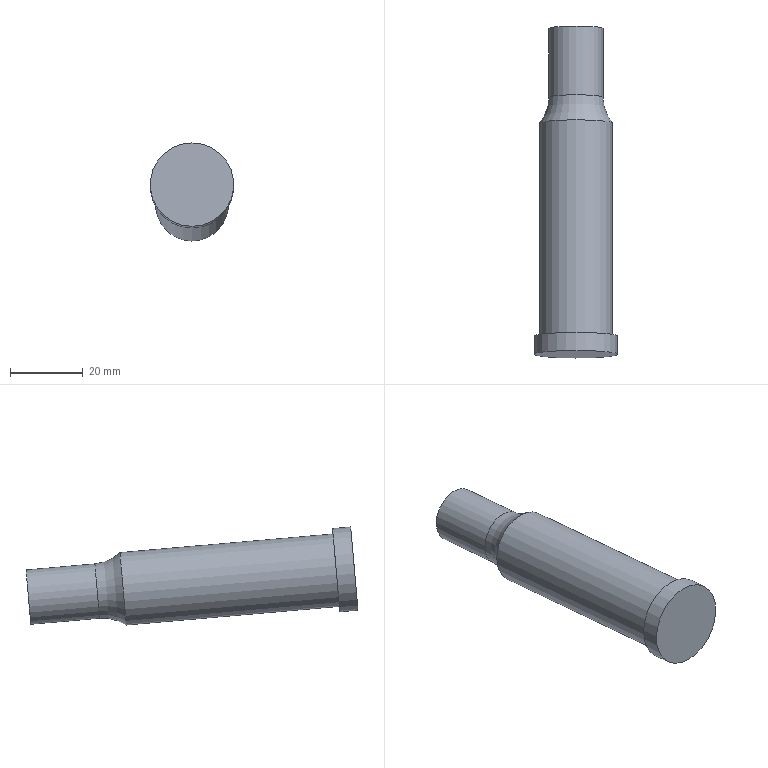Part | NX | features SPAS 20-80-18.00 2 | 1 solid | 7 faces | box 23 x 91.313 x 26.982 mm | volume 25479 mm3 | plane 3 | cylinder 3 | torus 1 | commonest cylinder face diameters 15 x1 20 x1 23 x1
STEP:
#1=CARTESIAN_POINT('',(-322.976,-54.628,-30.102));
#2=VERTEX_POINT('',#1);
#3=CARTESIAN_POINT('',(-322.976,-55.281,-37.573));
#4=DIRECTION('',(0.,0.9962,-0.08716));
#5=DIRECTION('',(0.,0.08716,0.9962));
#6=AXIS2_PLACEMENT_3D('',#3,#4,#5);
#7=CIRCLE('',#6,7.5);
#8=EDGE_CURVE('',#2,#2,#7,.F.);
#9=ORIENTED_EDGE('',*,*,#8,.F.);
#10=EDGE_LOOP('',(#9));
#11=FACE_BOUND('',#10,.T.);
#12=CARTESIAN_POINT('',(-322.976,-55.281,-37.573));
#13=DIRECTION('',(0.,0.9962,-0.08716));
#14=DIRECTION('',(0.,0.08716,0.9962));
#15=AXIS2_PLACEMENT_3D('',#12,#13,#14);
#16=PLANE('',#15);
#17=ADVANCED_FACE('',(#11),#16,.T.);
#18=CARTESIAN_POINT('',(-322.976,-74.863,-43.389));
#19=VERTEX_POINT('',#18);
#20=CARTESIAN_POINT('',(-322.976,-74.209,-35.917));
#21=DIRECTION('',(0.,-0.9962,0.08716));
#22=DIRECTION('',(0.,-0.08716,-0.9962));
#23=AXIS2_PLACEMENT_3D('',#20,#21,#22);
#24=CIRCLE('',#23,7.5);
#25=EDGE_CURVE('',#19,#19,#24,.F.);
#26=ORIENTED_EDGE('',*,*,#25,.T.);
#27=EDGE_LOOP('',(#26));
#28=FACE_BOUND('',#27,.T.);
#29=ORIENTED_EDGE('',*,*,#8,.T.);
#30=EDGE_LOOP('',(#29));
#31=FACE_BOUND('',#30,.T.);
#32=CARTESIAN_POINT('',(-322.976,-55.281,-37.573));
#33=DIRECTION('',(0.,-0.9962,0.08716));
#34=DIRECTION('',(0.,-0.08716,-0.9962));
#35=AXIS2_PLACEMENT_3D('',#32,#33,#34);
#36=CYLINDRICAL_SURFACE('',#35,7.5);
#37=ADVANCED_FACE('',(#28,#31),#36,.T.);
#38=CARTESIAN_POINT('',(-322.976,-139.086,-20.203));
#39=VERTEX_POINT('',#38);
#40=CARTESIAN_POINT('',(-322.976,-139.958,-30.165));
#41=DIRECTION('',(0.,0.9962,-0.08716));
#42=DIRECTION('',(0.,0.08716,0.9962));
#43=AXIS2_PLACEMENT_3D('',#40,#41,#42);
#44=CIRCLE('',#43,10.);
#45=EDGE_CURVE('',#39,#39,#44,.F.);
#46=ORIENTED_EDGE('',*,*,#45,.F.);
#47=EDGE_LOOP('',(#46));
#48=FACE_BOUND('',#47,.T.);
#49=CARTESIAN_POINT('',(-322.976,-80.469,-25.331));
#50=VERTEX_POINT('',#49);
#51=CARTESIAN_POINT('',(-322.976,-81.341,-35.293));
#52=DIRECTION('',(0.,0.9962,-0.08716));
#53=DIRECTION('',(0.,0.08716,0.9962));
#54=AXIS2_PLACEMENT_3D('',#51,#52,#53);
#55=CIRCLE('',#54,10.);
#56=EDGE_CURVE('',#50,#50,#55,.F.);
#57=ORIENTED_EDGE('',*,*,#56,.T.);
#58=EDGE_LOOP('',(#57));
#59=FACE_BOUND('',#58,.T.);
#60=CARTESIAN_POINT('',(-322.976,-78.552,-35.537));
#61=DIRECTION('',(0.,-0.9962,0.08716));
#62=DIRECTION('',(0.,-0.08716,-0.9962));
#63=AXIS2_PLACEMENT_3D('',#60,#61,#62);
#64=CYLINDRICAL_SURFACE('',#63,10.);
#65=ADVANCED_FACE('',(#48,#59),#64,.T.);
#66=CARTESIAN_POINT('',(-322.976,-145.941,-41.185));
#67=VERTEX_POINT('',#66);
#68=CARTESIAN_POINT('',(-322.976,-144.939,-29.729));
#69=DIRECTION('',(0.,-0.9962,0.08716));
#70=DIRECTION('',(0.,-0.08716,-0.9962));
#71=AXIS2_PLACEMENT_3D('',#68,#69,#70);
#72=CIRCLE('',#71,11.5);
#73=EDGE_CURVE('',#67,#67,#72,.F.);
#74=ORIENTED_EDGE('',*,*,#73,.F.);
#75=EDGE_LOOP('',(#74));
#76=FACE_BOUND('',#75,.T.);
#77=CARTESIAN_POINT('',(-322.976,-144.939,-29.729));
#78=DIRECTION('',(0.,-0.9962,0.08716));
#79=DIRECTION('',(0.,-0.08716,-0.9962));
#80=AXIS2_PLACEMENT_3D('',#77,#78,#79);
#81=PLANE('',#80);
#82=ADVANCED_FACE('',(#76),#81,.T.);
#83=ORIENTED_EDGE('',*,*,#45,.T.);
#84=EDGE_LOOP('',(#83));
#85=FACE_BOUND('',#84,.T.);
#86=CARTESIAN_POINT('',(-322.976,-138.956,-18.709));
#87=VERTEX_POINT('',#86);
#88=CARTESIAN_POINT('',(-322.976,-139.958,-30.165));
#89=DIRECTION('',(0.,0.9962,-0.08716));
#90=DIRECTION('',(0.,0.08716,0.9962));
#91=AXIS2_PLACEMENT_3D('',#88,#89,#90);
#92=CIRCLE('',#91,11.5);
#93=EDGE_CURVE('',#87,#87,#92,.F.);
#94=ORIENTED_EDGE('',*,*,#93,.F.);
#95=EDGE_LOOP('',(#94));
#96=FACE_BOUND('',#95,.T.);
#97=CARTESIAN_POINT('',(-322.976,-139.958,-30.165));
#98=DIRECTION('',(0.,0.9962,-0.08716));
#99=DIRECTION('',(0.,0.08716,0.9962));
#100=AXIS2_PLACEMENT_3D('',#97,#98,#99);
#101=PLANE('',#100);
#102=ADVANCED_FACE('',(#85,#96),#101,.T.);
#103=ORIENTED_EDGE('',*,*,#73,.T.);
#104=EDGE_LOOP('',(#103));
#105=FACE_BOUND('',#104,.T.);
#106=ORIENTED_EDGE('',*,*,#93,.T.);
#107=EDGE_LOOP('',(#106));
#108=FACE_BOUND('',#107,.T.);
#109=CARTESIAN_POINT('',(-322.976,-129.996,-31.037));
#110=DIRECTION('',(0.,-0.9962,0.08716));
#111=DIRECTION('',(0.,-0.08716,-0.9962));
#112=AXIS2_PLACEMENT_3D('',#109,#110,#111);
#113=CYLINDRICAL_SURFACE('',#112,11.5);
#114=ADVANCED_FACE('',(#105,#108),#113,.T.);
#115=ORIENTED_EDGE('',*,*,#25,.F.);
#116=EDGE_LOOP('',(#115));
#117=FACE_BOUND('',#116,.T.);
#118=ORIENTED_EDGE('',*,*,#56,.F.);
#119=EDGE_LOOP('',(#118));
#120=FACE_BOUND('',#119,.T.);
#121=CARTESIAN_POINT('',(-322.976,-74.209,-35.917));
#122=DIRECTION('',(0.,-0.9962,0.08716));
#123=DIRECTION('',(0.,-0.08716,-0.9962));
#124=AXIS2_PLACEMENT_3D('',#121,#122,#123);
#125=TOROIDAL_SURFACE('',#124,19.,11.5);
#126=ADVANCED_FACE('',(#117,#120),#125,.F.);
#127=CLOSED_SHELL('',(#17,#37,#65,#82,#102,#114,#126));
#128=MANIFOLD_SOLID_BREP('',#127);
#129=(LENGTH_UNIT()NAMED_UNIT(*)SI_UNIT(.MILLI.,.METRE.));
#130=UNCERTAINTY_MEASURE_WITH_UNIT(LENGTH_MEASURE(0.00001),#129,'','');
#131=(NAMED_UNIT(*)PLANE_ANGLE_UNIT()SI_UNIT($,.RADIAN.));
#132=(NAMED_UNIT(*)SI_UNIT($,.STERADIAN.)SOLID_ANGLE_UNIT());
#133=(GEOMETRIC_REPRESENTATION_CONTEXT(3)GLOBAL_UNCERTAINTY_ASSIGNED_CONTEXT((#130))GLOBAL_UNIT_ASSIGNED_CONTEXT((#129,#131,#132))REPRESENTATION_CONTEXT('',''));
#134=ADVANCED_BREP_SHAPE_REPRESENTATION('',(#128),#133);